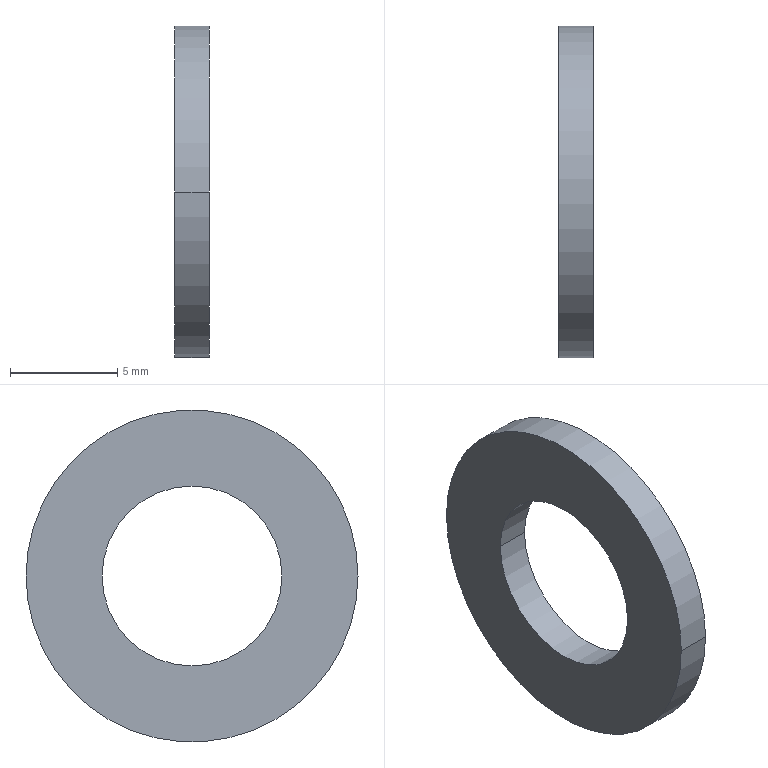Part | STEP file | KS B 1326 - 8x15.5 | 1 solid | 6 faces | box 1.6 x 15.5 x 15.5 mm | volume 213.239 mm3 | cylinder 4 | plane 2 | commonest cylinder face diameters 8.4 x2 15.5 x2
STEP:
#1=CARTESIAN_POINT('',(0.,0.,0.));
#2=DIRECTION('',(0.,0.,1.));
#3=DIRECTION('',(1.,0.,0.));
#4=AXIS2_PLACEMENT_3D('',#1,#2,#3);
#5=CARTESIAN_POINT('',(0.,-4.2,0.));
#6=VERTEX_POINT('',#5);
#7=CARTESIAN_POINT('',(1.6,-4.2,0.));
#8=VERTEX_POINT('',#7);
#9=CARTESIAN_POINT('',(0.,-4.2,0.));
#10=DIRECTION('',(1.,0.,0.));
#11=VECTOR('',#10,1.);
#12=LINE('',#9,#11);
#13=CARTESIAN_POINT('',(0.,0.,0.));
#14=DIRECTION('',(1.,0.,0.));
#15=DIRECTION('',(0.,-1.,0.));
#16=AXIS2_PLACEMENT_3D('',#13,#14,#15);
#17=CYLINDRICAL_SURFACE('',#16,4.2);
#18=CARTESIAN_POINT('',(6.283,0.));
#19=DIRECTION('',(0.,1.));
#20=VECTOR('',#19,1.);
#21=LINE('',#18,#20);
#22=(GEOMETRIC_REPRESENTATION_CONTEXT(2)PARAMETRIC_REPRESENTATION_CONTEXT()REPRESENTATION_CONTEXT('',''));
#23=DEFINITIONAL_REPRESENTATION('',(#21),#22);
#24=PCURVE('',#17,#23);
#25=CARTESIAN_POINT('',(0.,0.,0.));
#26=DIRECTION('',(1.,0.,0.));
#27=DIRECTION('',(0.,-1.,0.));
#28=AXIS2_PLACEMENT_3D('',#25,#26,#27);
#29=CYLINDRICAL_SURFACE('',#28,4.2);
#30=CARTESIAN_POINT('',(0.,0.));
#31=DIRECTION('',(0.,1.));
#32=VECTOR('',#31,1.);
#33=LINE('',#30,#32);
#34=(GEOMETRIC_REPRESENTATION_CONTEXT(2)PARAMETRIC_REPRESENTATION_CONTEXT()REPRESENTATION_CONTEXT('',''));
#35=DEFINITIONAL_REPRESENTATION('',(#33),#34);
#36=PCURVE('',#29,#35);
#37=SURFACE_CURVE('',#12,(#24,#36),.PCURVE_S1.);
#38=EDGE_CURVE('',#6,#8,#37,.T.);
#39=ORIENTED_EDGE('',*,*,#38,.T.);
#40=CARTESIAN_POINT('',(1.6,4.2,0.));
#41=VERTEX_POINT('',#40);
#42=CARTESIAN_POINT('',(1.6,0.,0.));
#43=DIRECTION('',(-1.,0.,0.));
#44=DIRECTION('',(0.,-1.,0.));
#45=AXIS2_PLACEMENT_3D('',#42,#43,#44);
#46=CIRCLE('',#45,4.2);
#47=CARTESIAN_POINT('',(6.283,1.6));
#48=DIRECTION('',(-1.,0.));
#49=VECTOR('',#48,1.);
#50=LINE('',#47,#49);
#51=(GEOMETRIC_REPRESENTATION_CONTEXT(2)PARAMETRIC_REPRESENTATION_CONTEXT()REPRESENTATION_CONTEXT('',''));
#52=DEFINITIONAL_REPRESENTATION('',(#50),#51);
#53=PCURVE('',#17,#52);
#54=CARTESIAN_POINT('',(1.6,0.,0.));
#55=DIRECTION('',(-1.,0.,0.));
#56=DIRECTION('',(0.,0.,1.));
#57=AXIS2_PLACEMENT_3D('',#54,#55,#56);
#58=PLANE('',#57);
#59=CARTESIAN_POINT('',(0.,0.));
#60=DIRECTION('',(0.,-1.));
#61=AXIS2_PLACEMENT_2D('',#59,#60);
#62=CIRCLE('',#61,4.2);
#63=(GEOMETRIC_REPRESENTATION_CONTEXT(2)PARAMETRIC_REPRESENTATION_CONTEXT()REPRESENTATION_CONTEXT('',''));
#64=DEFINITIONAL_REPRESENTATION('',(#62),#63);
#65=PCURVE('',#58,#64);
#66=SURFACE_CURVE('',#46,(#53,#65),.PCURVE_S1.);
#67=EDGE_CURVE('',#8,#41,#66,.T.);
#68=ORIENTED_EDGE('',*,*,#67,.T.);
#69=CARTESIAN_POINT('',(0.,4.2,0.));
#70=VERTEX_POINT('',#69);
#71=CARTESIAN_POINT('',(0.,4.2,0.));
#72=DIRECTION('',(1.,0.,0.));
#73=VECTOR('',#72,1.);
#74=LINE('',#71,#73);
#75=CARTESIAN_POINT('',(3.142,0.));
#76=DIRECTION('',(0.,1.));
#77=VECTOR('',#76,1.);
#78=LINE('',#75,#77);
#79=(GEOMETRIC_REPRESENTATION_CONTEXT(2)PARAMETRIC_REPRESENTATION_CONTEXT()REPRESENTATION_CONTEXT('',''));
#80=DEFINITIONAL_REPRESENTATION('',(#78),#79);
#81=PCURVE('',#17,#80);
#82=CARTESIAN_POINT('',(3.142,0.));
#83=DIRECTION('',(0.,1.));
#84=VECTOR('',#83,1.);
#85=LINE('',#82,#84);
#86=(GEOMETRIC_REPRESENTATION_CONTEXT(2)PARAMETRIC_REPRESENTATION_CONTEXT()REPRESENTATION_CONTEXT('',''));
#87=DEFINITIONAL_REPRESENTATION('',(#85),#86);
#88=PCURVE('',#29,#87);
#89=SURFACE_CURVE('',#74,(#81,#88),.PCURVE_S1.);
#90=EDGE_CURVE('',#70,#41,#89,.T.);
#91=ORIENTED_EDGE('',*,*,#90,.F.);
#92=CARTESIAN_POINT('',(0.,0.,0.));
#93=DIRECTION('',(1.,0.,0.));
#94=DIRECTION('',(0.,-1.,0.));
#95=AXIS2_PLACEMENT_3D('',#92,#93,#94);
#96=CIRCLE('',#95,4.2);
#97=CARTESIAN_POINT('',(0.,0.));
#98=DIRECTION('',(1.,0.));
#99=VECTOR('',#98,1.);
#100=LINE('',#97,#99);
#101=(GEOMETRIC_REPRESENTATION_CONTEXT(2)PARAMETRIC_REPRESENTATION_CONTEXT()REPRESENTATION_CONTEXT('',''));
#102=DEFINITIONAL_REPRESENTATION('',(#100),#101);
#103=PCURVE('',#17,#102);
#104=CARTESIAN_POINT('',(0.,0.,0.));
#105=DIRECTION('',(-1.,0.,0.));
#106=DIRECTION('',(0.,0.,1.));
#107=AXIS2_PLACEMENT_3D('',#104,#105,#106);
#108=PLANE('',#107);
#109=CARTESIAN_POINT('',(0.,-4.2));
#110=CARTESIAN_POINT('',(-7.275,-4.2));
#111=CARTESIAN_POINT('',(-3.637,2.1));
#112=CARTESIAN_POINT('',(0.,8.4));
#113=CARTESIAN_POINT('',(3.637,2.1));
#114=CARTESIAN_POINT('',(7.275,-4.2));
#115=CARTESIAN_POINT('',(0.,-4.2));
#116=(BOUNDED_CURVE()B_SPLINE_CURVE(2,(#109,#110,#111,#112,#113,#114,#115),.UNSPECIFIED.,.T.,.F.)B_SPLINE_CURVE_WITH_KNOTS((1,2,2,2,2,1),(-2.094,0.,2.094,4.189,6.283,8.378),.UNSPECIFIED.)CURVE()GEOMETRIC_REPRESENTATION_ITEM()RATIONAL_B_SPLINE_CURVE((1.,0.5,1.,0.5,1.,0.5,1.))REPRESENTATION_ITEM(''));
#117=(GEOMETRIC_REPRESENTATION_CONTEXT(2)PARAMETRIC_REPRESENTATION_CONTEXT()REPRESENTATION_CONTEXT('',''));
#118=DEFINITIONAL_REPRESENTATION('',(#116),#117);
#119=PCURVE('',#108,#118);
#120=SURFACE_CURVE('',#96,(#103,#119),.PCURVE_S1.);
#121=EDGE_CURVE('',#70,#6,#120,.T.);
#122=ORIENTED_EDGE('',*,*,#121,.T.);
#123=EDGE_LOOP('',(#39,#68,#91,#122));
#124=FACE_BOUND('',#123,.F.);
#125=ADVANCED_FACE('',(#124),#17,.F.);
#126=CARTESIAN_POINT('',(0.,7.75,0.));
#127=VERTEX_POINT('',#126);
#128=CARTESIAN_POINT('',(0.,-7.75,0.));
#129=VERTEX_POINT('',#128);
#130=CARTESIAN_POINT('',(0.,0.,0.));
#131=DIRECTION('',(-1.,0.,0.));
#132=DIRECTION('',(0.,-1.,0.));
#133=AXIS2_PLACEMENT_3D('',#130,#131,#132);
#134=CIRCLE('',#133,7.75);
#135=CARTESIAN_POINT('',(0.,0.,0.));
#136=DIRECTION('',(1.,0.,0.));
#137=DIRECTION('',(0.,-1.,0.));
#138=AXIS2_PLACEMENT_3D('',#135,#136,#137);
#139=CYLINDRICAL_SURFACE('',#138,7.75);
#140=CARTESIAN_POINT('',(6.283,0.));
#141=DIRECTION('',(-1.,0.));
#142=VECTOR('',#141,1.);
#143=LINE('',#140,#142);
#144=(GEOMETRIC_REPRESENTATION_CONTEXT(2)PARAMETRIC_REPRESENTATION_CONTEXT()REPRESENTATION_CONTEXT('',''));
#145=DEFINITIONAL_REPRESENTATION('',(#143),#144);
#146=PCURVE('',#139,#145);
#147=CARTESIAN_POINT('',(0.,0.));
#148=DIRECTION('',(0.,-1.));
#149=AXIS2_PLACEMENT_2D('',#147,#148);
#150=CIRCLE('',#149,7.75);
#151=(GEOMETRIC_REPRESENTATION_CONTEXT(2)PARAMETRIC_REPRESENTATION_CONTEXT()REPRESENTATION_CONTEXT('',''));
#152=DEFINITIONAL_REPRESENTATION('',(#150),#151);
#153=PCURVE('',#108,#152);
#154=SURFACE_CURVE('',#134,(#146,#153),.PCURVE_S1.);
#155=EDGE_CURVE('',#127,#129,#154,.T.);
#156=ORIENTED_EDGE('',*,*,#155,.F.);
#157=CARTESIAN_POINT('',(1.6,7.75,0.));
#158=VERTEX_POINT('',#157);
#159=CARTESIAN_POINT('',(0.,7.75,0.));
#160=DIRECTION('',(1.,0.,0.));
#161=VECTOR('',#160,1.);
#162=LINE('',#159,#161);
#163=CARTESIAN_POINT('',(3.142,0.));
#164=DIRECTION('',(0.,1.));
#165=VECTOR('',#164,1.);
#166=LINE('',#163,#165);
#167=(GEOMETRIC_REPRESENTATION_CONTEXT(2)PARAMETRIC_REPRESENTATION_CONTEXT()REPRESENTATION_CONTEXT('',''));
#168=DEFINITIONAL_REPRESENTATION('',(#166),#167);
#169=PCURVE('',#139,#168);
#170=CARTESIAN_POINT('',(0.,0.,0.));
#171=DIRECTION('',(1.,0.,0.));
#172=DIRECTION('',(0.,-1.,0.));
#173=AXIS2_PLACEMENT_3D('',#170,#171,#172);
#174=CYLINDRICAL_SURFACE('',#173,7.75);
#175=CARTESIAN_POINT('',(3.142,0.));
#176=DIRECTION('',(0.,1.));
#177=VECTOR('',#176,1.);
#178=LINE('',#175,#177);
#179=(GEOMETRIC_REPRESENTATION_CONTEXT(2)PARAMETRIC_REPRESENTATION_CONTEXT()REPRESENTATION_CONTEXT('',''));
#180=DEFINITIONAL_REPRESENTATION('',(#178),#179);
#181=PCURVE('',#174,#180);
#182=SURFACE_CURVE('',#162,(#169,#181),.PCURVE_S1.);
#183=EDGE_CURVE('',#127,#158,#182,.T.);
#184=ORIENTED_EDGE('',*,*,#183,.T.);
#185=CARTESIAN_POINT('',(1.6,-7.75,0.));
#186=VERTEX_POINT('',#185);
#187=CARTESIAN_POINT('',(1.6,0.,0.));
#188=DIRECTION('',(-1.,0.,0.));
#189=DIRECTION('',(0.,-1.,0.));
#190=AXIS2_PLACEMENT_3D('',#187,#188,#189);
#191=CIRCLE('',#190,7.75);
#192=CARTESIAN_POINT('',(6.283,1.6));
#193=DIRECTION('',(-1.,0.));
#194=VECTOR('',#193,1.);
#195=LINE('',#192,#194);
#196=(GEOMETRIC_REPRESENTATION_CONTEXT(2)PARAMETRIC_REPRESENTATION_CONTEXT()REPRESENTATION_CONTEXT('',''));
#197=DEFINITIONAL_REPRESENTATION('',(#195),#196);
#198=PCURVE('',#139,#197);
#199=CARTESIAN_POINT('',(0.,0.));
#200=DIRECTION('',(0.,-1.));
#201=AXIS2_PLACEMENT_2D('',#199,#200);
#202=CIRCLE('',#201,7.75);
#203=(GEOMETRIC_REPRESENTATION_CONTEXT(2)PARAMETRIC_REPRESENTATION_CONTEXT()REPRESENTATION_CONTEXT('',''));
#204=DEFINITIONAL_REPRESENTATION('',(#202),#203);
#205=PCURVE('',#58,#204);
#206=SURFACE_CURVE('',#191,(#198,#205),.PCURVE_S1.);
#207=EDGE_CURVE('',#158,#186,#206,.T.);
#208=ORIENTED_EDGE('',*,*,#207,.T.);
#209=CARTESIAN_POINT('',(0.,-7.75,0.));
#210=DIRECTION('',(1.,0.,0.));
#211=VECTOR('',#210,1.);
#212=LINE('',#209,#211);
#213=CARTESIAN_POINT('',(0.,0.));
#214=DIRECTION('',(0.,1.));
#215=VECTOR('',#214,1.);
#216=LINE('',#213,#215);
#217=(GEOMETRIC_REPRESENTATION_CONTEXT(2)PARAMETRIC_REPRESENTATION_CONTEXT()REPRESENTATION_CONTEXT('',''));
#218=DEFINITIONAL_REPRESENTATION('',(#216),#217);
#219=PCURVE('',#139,#218);
#220=CARTESIAN_POINT('',(6.283,0.));
#221=DIRECTION('',(0.,1.));
#222=VECTOR('',#221,1.);
#223=LINE('',#220,#222);
#224=(GEOMETRIC_REPRESENTATION_CONTEXT(2)PARAMETRIC_REPRESENTATION_CONTEXT()REPRESENTATION_CONTEXT('',''));
#225=DEFINITIONAL_REPRESENTATION('',(#223),#224);
#226=PCURVE('',#174,#225);
#227=SURFACE_CURVE('',#212,(#219,#226),.PCURVE_S1.);
#228=EDGE_CURVE('',#129,#186,#227,.T.);
#229=ORIENTED_EDGE('',*,*,#228,.F.);
#230=EDGE_LOOP('',(#156,#184,#208,#229));
#231=FACE_BOUND('',#230,.T.);
#232=ADVANCED_FACE('',(#231),#139,.T.);
#233=CARTESIAN_POINT('',(0.,0.,0.));
#234=DIRECTION('',(1.,0.,0.));
#235=DIRECTION('',(0.,-1.,0.));
#236=AXIS2_PLACEMENT_3D('',#233,#234,#235);
#237=CIRCLE('',#236,4.2);
#238=CARTESIAN_POINT('',(0.,-4.2));
#239=CARTESIAN_POINT('',(-7.275,-4.2));
#240=CARTESIAN_POINT('',(-3.637,2.1));
#241=CARTESIAN_POINT('',(0.,8.4));
#242=CARTESIAN_POINT('',(3.637,2.1));
#243=CARTESIAN_POINT('',(7.275,-4.2));
#244=CARTESIAN_POINT('',(0.,-4.2));
#245=(BOUNDED_CURVE()B_SPLINE_CURVE(2,(#238,#239,#240,#241,#242,#243,#244),.UNSPECIFIED.,.T.,.F.)B_SPLINE_CURVE_WITH_KNOTS((1,2,2,2,2,1),(-2.094,0.,2.094,4.189,6.283,8.378),.UNSPECIFIED.)CURVE()GEOMETRIC_REPRESENTATION_ITEM()RATIONAL_B_SPLINE_CURVE((1.,0.5,1.,0.5,1.,0.5,1.))REPRESENTATION_ITEM(''));
#246=(GEOMETRIC_REPRESENTATION_CONTEXT(2)PARAMETRIC_REPRESENTATION_CONTEXT()REPRESENTATION_CONTEXT('',''));
#247=DEFINITIONAL_REPRESENTATION('',(#245),#246);
#248=PCURVE('',#108,#247);
#249=CARTESIAN_POINT('',(0.,0.));
#250=DIRECTION('',(1.,0.));
#251=VECTOR('',#250,1.);
#252=LINE('',#249,#251);
#253=(GEOMETRIC_REPRESENTATION_CONTEXT(2)PARAMETRIC_REPRESENTATION_CONTEXT()REPRESENTATION_CONTEXT('',''));
#254=DEFINITIONAL_REPRESENTATION('',(#252),#253);
#255=PCURVE('',#29,#254);
#256=SURFACE_CURVE('',#237,(#248,#255),.PCURVE_S1.);
#257=EDGE_CURVE('',#6,#70,#256,.T.);
#258=ORIENTED_EDGE('',*,*,#257,.T.);
#259=ORIENTED_EDGE('',*,*,#121,.T.);
#260=EDGE_LOOP('',(#258,#259));
#261=FACE_BOUND('',#260,.T.);
#262=CARTESIAN_POINT('',(0.,0.,0.));
#263=DIRECTION('',(-1.,0.,0.));
#264=DIRECTION('',(0.,-1.,0.));
#265=AXIS2_PLACEMENT_3D('',#262,#263,#264);
#266=CIRCLE('',#265,7.75);
#267=CARTESIAN_POINT('',(0.,0.));
#268=DIRECTION('',(0.,-1.));
#269=AXIS2_PLACEMENT_2D('',#267,#268);
#270=CIRCLE('',#269,7.75);
#271=(GEOMETRIC_REPRESENTATION_CONTEXT(2)PARAMETRIC_REPRESENTATION_CONTEXT()REPRESENTATION_CONTEXT('',''));
#272=DEFINITIONAL_REPRESENTATION('',(#270),#271);
#273=PCURVE('',#108,#272);
#274=CARTESIAN_POINT('',(6.283,0.));
#275=DIRECTION('',(-1.,0.));
#276=VECTOR('',#275,1.);
#277=LINE('',#274,#276);
#278=(GEOMETRIC_REPRESENTATION_CONTEXT(2)PARAMETRIC_REPRESENTATION_CONTEXT()REPRESENTATION_CONTEXT('',''));
#279=DEFINITIONAL_REPRESENTATION('',(#277),#278);
#280=PCURVE('',#174,#279);
#281=SURFACE_CURVE('',#266,(#273,#280),.PCURVE_S1.);
#282=EDGE_CURVE('',#129,#127,#281,.T.);
#283=ORIENTED_EDGE('',*,*,#282,.T.);
#284=ORIENTED_EDGE('',*,*,#155,.T.);
#285=EDGE_LOOP('',(#283,#284));
#286=FACE_BOUND('',#285,.T.);
#287=ADVANCED_FACE('',(#261,#286),#108,.T.);
#288=ORIENTED_EDGE('',*,*,#67,.T.);
#289=CARTESIAN_POINT('',(1.6,0.,0.));
#290=DIRECTION('',(-1.,0.,0.));
#291=DIRECTION('',(0.,-1.,0.));
#292=AXIS2_PLACEMENT_3D('',#289,#290,#291);
#293=CIRCLE('',#292,4.2);
#294=CARTESIAN_POINT('',(0.,0.));
#295=DIRECTION('',(0.,-1.));
#296=AXIS2_PLACEMENT_2D('',#294,#295);
#297=CIRCLE('',#296,4.2);
#298=(GEOMETRIC_REPRESENTATION_CONTEXT(2)PARAMETRIC_REPRESENTATION_CONTEXT()REPRESENTATION_CONTEXT('',''));
#299=DEFINITIONAL_REPRESENTATION('',(#297),#298);
#300=PCURVE('',#58,#299);
#301=CARTESIAN_POINT('',(6.283,1.6));
#302=DIRECTION('',(-1.,0.));
#303=VECTOR('',#302,1.);
#304=LINE('',#301,#303);
#305=(GEOMETRIC_REPRESENTATION_CONTEXT(2)PARAMETRIC_REPRESENTATION_CONTEXT()REPRESENTATION_CONTEXT('',''));
#306=DEFINITIONAL_REPRESENTATION('',(#304),#305);
#307=PCURVE('',#29,#306);
#308=SURFACE_CURVE('',#293,(#300,#307),.PCURVE_S1.);
#309=EDGE_CURVE('',#41,#8,#308,.T.);
#310=ORIENTED_EDGE('',*,*,#309,.T.);
#311=EDGE_LOOP('',(#288,#310));
#312=FACE_BOUND('',#311,.T.);
#313=CARTESIAN_POINT('',(1.6,0.,0.));
#314=DIRECTION('',(-1.,0.,0.));
#315=DIRECTION('',(0.,-1.,0.));
#316=AXIS2_PLACEMENT_3D('',#313,#314,#315);
#317=CIRCLE('',#316,7.75);
#318=CARTESIAN_POINT('',(0.,0.));
#319=DIRECTION('',(0.,-1.));
#320=AXIS2_PLACEMENT_2D('',#318,#319);
#321=CIRCLE('',#320,7.75);
#322=(GEOMETRIC_REPRESENTATION_CONTEXT(2)PARAMETRIC_REPRESENTATION_CONTEXT()REPRESENTATION_CONTEXT('',''));
#323=DEFINITIONAL_REPRESENTATION('',(#321),#322);
#324=PCURVE('',#58,#323);
#325=CARTESIAN_POINT('',(6.283,1.6));
#326=DIRECTION('',(-1.,0.));
#327=VECTOR('',#326,1.);
#328=LINE('',#325,#327);
#329=(GEOMETRIC_REPRESENTATION_CONTEXT(2)PARAMETRIC_REPRESENTATION_CONTEXT()REPRESENTATION_CONTEXT('',''));
#330=DEFINITIONAL_REPRESENTATION('',(#328),#329);
#331=PCURVE('',#174,#330);
#332=SURFACE_CURVE('',#317,(#324,#331),.PCURVE_S1.);
#333=EDGE_CURVE('',#186,#158,#332,.T.);
#334=ORIENTED_EDGE('',*,*,#333,.F.);
#335=ORIENTED_EDGE('',*,*,#207,.F.);
#336=EDGE_LOOP('',(#334,#335));
#337=FACE_BOUND('',#336,.T.);
#338=ADVANCED_FACE('',(#312,#337),#58,.F.);
#339=ORIENTED_EDGE('',*,*,#183,.F.);
#340=ORIENTED_EDGE('',*,*,#282,.F.);
#341=ORIENTED_EDGE('',*,*,#228,.T.);
#342=ORIENTED_EDGE('',*,*,#333,.T.);
#343=EDGE_LOOP('',(#339,#340,#341,#342));
#344=FACE_BOUND('',#343,.T.);
#345=ADVANCED_FACE('',(#344),#174,.T.);
#346=ORIENTED_EDGE('',*,*,#309,.T.);
#347=ORIENTED_EDGE('',*,*,#38,.F.);
#348=ORIENTED_EDGE('',*,*,#257,.T.);
#349=ORIENTED_EDGE('',*,*,#90,.T.);
#350=EDGE_LOOP('',(#346,#347,#348,#349));
#351=FACE_BOUND('',#350,.F.);
#352=ADVANCED_FACE('',(#351),#29,.F.);
#353=CLOSED_SHELL('',(#125,#232,#287,#338,#345,#352));
#354=MANIFOLD_SOLID_BREP('',#353);
#355=(LENGTH_UNIT()NAMED_UNIT(*)SI_UNIT(.MILLI.,.METRE.));
#356=UNCERTAINTY_MEASURE_WITH_UNIT(LENGTH_MEASURE(0.0000001),#355,'','');
#357=(NAMED_UNIT(*)PLANE_ANGLE_UNIT()SI_UNIT($,.RADIAN.));
#358=(NAMED_UNIT(*)SI_UNIT($,.STERADIAN.)SOLID_ANGLE_UNIT());
#359=(GEOMETRIC_REPRESENTATION_CONTEXT(3)GLOBAL_UNCERTAINTY_ASSIGNED_CONTEXT((#356))GLOBAL_UNIT_ASSIGNED_CONTEXT((#355,#357,#358))REPRESENTATION_CONTEXT('',''));
#360=ADVANCED_BREP_SHAPE_REPRESENTATION('',(#4,#354),#359);